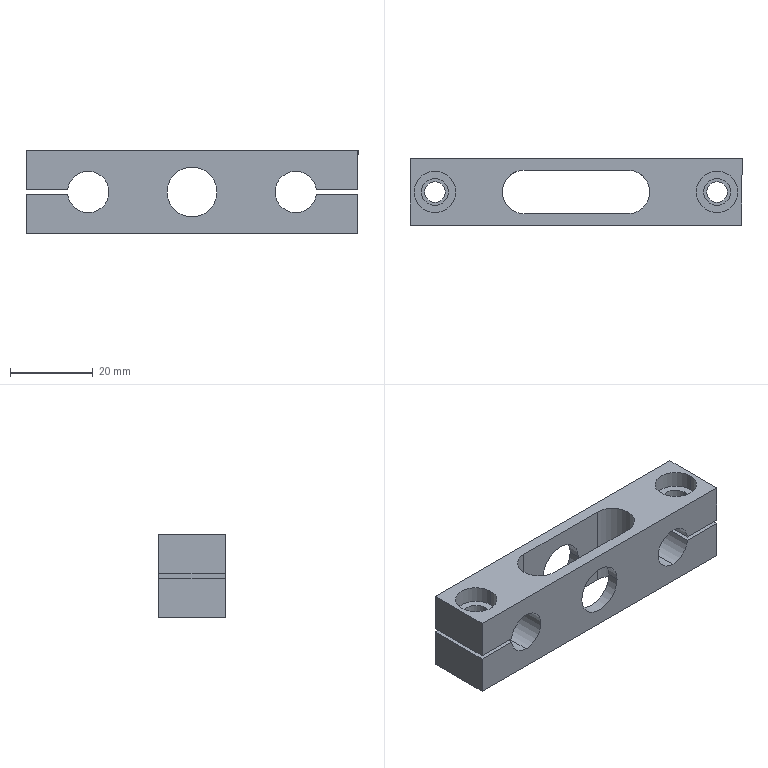Part | SolidWorks | features ICE 5, Extrusion 1, HoleWzd 1 | 1 solid | 41 faces | box 80 x 16 x 20 mm | volume 13796 mm3 | cylinder 25 | plane 16 | commonest cylinder face diameters 10 x10 5 x4 6.5 x4 12 x4 10.5 x3
STEP:
#1=CARTESIAN_POINT('',(-29.662,6.461,16.));
#2=VERTEX_POINT('',#1);
#3=CARTESIAN_POINT('',(-19.662,6.461,16.));
#4=VERTEX_POINT('',#3);
#5=CARTESIAN_POINT('',(-24.662,6.461,16.));
#6=DIRECTION('',(0.,0.,1.));
#7=DIRECTION('',(1.,0.,0.));
#8=AXIS2_PLACEMENT_3D('',#5,#6,#7);
#9=CIRCLE('',#8,5.);
#10=EDGE_CURVE('',#2,#4,#9,.T.);
#11=ORIENTED_EDGE('',*,*,#10,.F.);
#12=CARTESIAN_POINT('',(-29.662,6.461,20.));
#13=VERTEX_POINT('',#12);
#14=CARTESIAN_POINT('',(-29.662,6.461,16.));
#15=DIRECTION('',(0.,0.,1.));
#16=VECTOR('',#15,1000.);
#17=LINE('',#14,#16);
#18=EDGE_CURVE('',#2,#13,#17,.T.);
#19=ORIENTED_EDGE('',*,*,#18,.T.);
#20=CARTESIAN_POINT('',(-19.662,6.461,20.));
#21=VERTEX_POINT('',#20);
#22=CARTESIAN_POINT('',(-24.662,6.461,20.));
#23=DIRECTION('',(0.,0.,1.));
#24=DIRECTION('',(1.,0.,0.));
#25=AXIS2_PLACEMENT_3D('',#22,#23,#24);
#26=CIRCLE('',#25,5.);
#27=EDGE_CURVE('',#13,#21,#26,.T.);
#28=ORIENTED_EDGE('',*,*,#27,.T.);
#29=CARTESIAN_POINT('',(-19.662,6.461,16.));
#30=DIRECTION('',(0.,0.,1.));
#31=VECTOR('',#30,1000.);
#32=LINE('',#29,#31);
#33=EDGE_CURVE('',#4,#21,#32,.T.);
#34=ORIENTED_EDGE('',*,*,#33,.F.);
#35=EDGE_LOOP('',(#11,#19,#28,#34));
#36=FACE_OUTER_BOUND('',#35,.T.);
#37=CARTESIAN_POINT('',(-24.662,6.461,16.));
#38=DIRECTION('',(0.,0.,1.));
#39=DIRECTION('',(1.,0.,0.));
#40=AXIS2_PLACEMENT_3D('',#37,#38,#39);
#41=CYLINDRICAL_SURFACE('',#40,5.);
#42=ADVANCED_FACE('',(#36),#41,.F.);
#43=CARTESIAN_POINT('',(38.338,6.461,16.));
#44=VERTEX_POINT('',#43);
#45=CARTESIAN_POINT('',(48.338,6.461,16.));
#46=VERTEX_POINT('',#45);
#47=CARTESIAN_POINT('',(43.338,6.461,16.));
#48=DIRECTION('',(0.,0.,1.));
#49=DIRECTION('',(1.,0.,0.));
#50=AXIS2_PLACEMENT_3D('',#47,#48,#49);
#51=CIRCLE('',#50,5.);
#52=EDGE_CURVE('',#44,#46,#51,.T.);
#53=ORIENTED_EDGE('',*,*,#52,.F.);
#54=CARTESIAN_POINT('',(38.338,6.461,20.));
#55=VERTEX_POINT('',#54);
#56=CARTESIAN_POINT('',(38.338,6.461,16.));
#57=DIRECTION('',(0.,0.,1.));
#58=VECTOR('',#57,1000.);
#59=LINE('',#56,#58);
#60=EDGE_CURVE('',#44,#55,#59,.T.);
#61=ORIENTED_EDGE('',*,*,#60,.T.);
#62=CARTESIAN_POINT('',(48.338,6.461,20.));
#63=VERTEX_POINT('',#62);
#64=CARTESIAN_POINT('',(43.338,6.461,20.));
#65=DIRECTION('',(0.,0.,1.));
#66=DIRECTION('',(1.,0.,0.));
#67=AXIS2_PLACEMENT_3D('',#64,#65,#66);
#68=CIRCLE('',#67,5.);
#69=EDGE_CURVE('',#55,#63,#68,.T.);
#70=ORIENTED_EDGE('',*,*,#69,.T.);
#71=CARTESIAN_POINT('',(48.338,6.461,16.));
#72=DIRECTION('',(0.,0.,1.));
#73=VECTOR('',#72,1000.);
#74=LINE('',#71,#73);
#75=EDGE_CURVE('',#46,#63,#74,.T.);
#76=ORIENTED_EDGE('',*,*,#75,.F.);
#77=EDGE_LOOP('',(#53,#61,#70,#76));
#78=FACE_OUTER_BOUND('',#77,.T.);
#79=CARTESIAN_POINT('',(43.338,6.461,16.));
#80=DIRECTION('',(0.,0.,1.));
#81=DIRECTION('',(1.,0.,0.));
#82=AXIS2_PLACEMENT_3D('',#79,#80,#81);
#83=CYLINDRICAL_SURFACE('',#82,5.);
#84=ADVANCED_FACE('',(#78),#83,.F.);
#85=CARTESIAN_POINT('',(45.838,6.461,0.));
#86=VERTEX_POINT('',#85);
#87=CARTESIAN_POINT('',(40.838,6.461,0.));
#88=VERTEX_POINT('',#87);
#89=CARTESIAN_POINT('',(43.338,6.461,0.));
#90=DIRECTION('',(0.,0.,-1.));
#91=DIRECTION('',(-1.,0.,0.));
#92=AXIS2_PLACEMENT_3D('',#89,#90,#91);
#93=CIRCLE('',#92,2.5);
#94=EDGE_CURVE('',#86,#88,#93,.T.);
#95=ORIENTED_EDGE('',*,*,#94,.T.);
#96=CARTESIAN_POINT('',(40.838,6.461,9.5));
#97=VERTEX_POINT('',#96);
#98=CARTESIAN_POINT('',(40.838,6.461,9.5));
#99=DIRECTION('',(0.,0.,1.));
#100=VECTOR('',#99,1000.);
#101=LINE('',#98,#100);
#102=EDGE_CURVE('',#88,#97,#101,.T.);
#103=ORIENTED_EDGE('',*,*,#102,.T.);
#104=CARTESIAN_POINT('',(45.838,6.461,9.5));
#105=VERTEX_POINT('',#104);
#106=CARTESIAN_POINT('',(43.338,6.461,9.5));
#107=DIRECTION('',(0.,0.,1.));
#108=DIRECTION('',(1.,0.,0.));
#109=AXIS2_PLACEMENT_3D('',#106,#107,#108);
#110=CIRCLE('',#109,2.5);
#111=EDGE_CURVE('',#97,#105,#110,.T.);
#112=ORIENTED_EDGE('',*,*,#111,.T.);
#113=CARTESIAN_POINT('',(45.838,6.461,9.5));
#114=DIRECTION('',(0.,0.,1.));
#115=VECTOR('',#114,1000.);
#116=LINE('',#113,#115);
#117=EDGE_CURVE('',#86,#105,#116,.T.);
#118=ORIENTED_EDGE('',*,*,#117,.F.);
#119=EDGE_LOOP('',(#95,#103,#112,#118));
#120=FACE_OUTER_BOUND('',#119,.T.);
#121=CARTESIAN_POINT('',(43.338,6.461,9.5));
#122=DIRECTION('',(0.,0.,1.));
#123=DIRECTION('',(1.,0.,0.));
#124=AXIS2_PLACEMENT_3D('',#121,#122,#123);
#125=CYLINDRICAL_SURFACE('',#124,2.5);
#126=ADVANCED_FACE('',(#120),#125,.F.);
#127=CARTESIAN_POINT('',(-22.162,6.461,0.));
#128=VERTEX_POINT('',#127);
#129=CARTESIAN_POINT('',(-27.162,6.461,0.));
#130=VERTEX_POINT('',#129);
#131=CARTESIAN_POINT('',(-24.662,6.461,0.));
#132=DIRECTION('',(0.,0.,-1.));
#133=DIRECTION('',(-1.,0.,0.));
#134=AXIS2_PLACEMENT_3D('',#131,#132,#133);
#135=CIRCLE('',#134,2.5);
#136=EDGE_CURVE('',#128,#130,#135,.T.);
#137=ORIENTED_EDGE('',*,*,#136,.T.);
#138=CARTESIAN_POINT('',(-27.162,6.461,9.5));
#139=VERTEX_POINT('',#138);
#140=CARTESIAN_POINT('',(-27.162,6.461,9.5));
#141=DIRECTION('',(0.,0.,1.));
#142=VECTOR('',#141,1000.);
#143=LINE('',#140,#142);
#144=EDGE_CURVE('',#130,#139,#143,.T.);
#145=ORIENTED_EDGE('',*,*,#144,.T.);
#146=CARTESIAN_POINT('',(-22.162,6.461,9.5));
#147=VERTEX_POINT('',#146);
#148=CARTESIAN_POINT('',(-24.662,6.461,9.5));
#149=DIRECTION('',(0.,0.,1.));
#150=DIRECTION('',(1.,0.,0.));
#151=AXIS2_PLACEMENT_3D('',#148,#149,#150);
#152=CIRCLE('',#151,2.5);
#153=EDGE_CURVE('',#139,#147,#152,.T.);
#154=ORIENTED_EDGE('',*,*,#153,.T.);
#155=CARTESIAN_POINT('',(-22.162,6.461,9.5));
#156=DIRECTION('',(0.,0.,1.));
#157=VECTOR('',#156,1000.);
#158=LINE('',#155,#157);
#159=EDGE_CURVE('',#128,#147,#158,.T.);
#160=ORIENTED_EDGE('',*,*,#159,.F.);
#161=EDGE_LOOP('',(#137,#145,#154,#160));
#162=FACE_OUTER_BOUND('',#161,.T.);
#163=CARTESIAN_POINT('',(-24.662,6.461,9.5));
#164=DIRECTION('',(0.,0.,1.));
#165=DIRECTION('',(1.,0.,0.));
#166=AXIS2_PLACEMENT_3D('',#163,#164,#165);
#167=CYLINDRICAL_SURFACE('',#166,2.5);
#168=ADVANCED_FACE('',(#162),#167,.F.);
#169=CARTESIAN_POINT('',(15.338,1.211,10.));
#170=VERTEX_POINT('',#169);
#171=CARTESIAN_POINT('',(3.338,1.211,10.));
#172=VERTEX_POINT('',#171);
#173=CARTESIAN_POINT('',(9.338,1.211,10.));
#174=DIRECTION('',(0.,1.,0.));
#175=DIRECTION('',(0.,0.,1.));
#176=AXIS2_PLACEMENT_3D('',#173,#174,#175);
#177=CIRCLE('',#176,6.);
#178=EDGE_CURVE('',#170,#172,#177,.T.);
#179=ORIENTED_EDGE('',*,*,#178,.T.);
#180=CARTESIAN_POINT('',(3.338,-1.539,10.));
#181=VERTEX_POINT('',#180);
#182=CARTESIAN_POINT('',(3.338,28.211,10.));
#183=DIRECTION('',(0.,-1.,0.));
#184=VECTOR('',#183,1000.);
#185=LINE('',#182,#184);
#186=EDGE_CURVE('',#172,#181,#185,.T.);
#187=ORIENTED_EDGE('',*,*,#186,.T.);
#188=CARTESIAN_POINT('',(15.338,-1.539,10.));
#189=VERTEX_POINT('',#188);
#190=CARTESIAN_POINT('',(9.338,-1.539,10.));
#191=DIRECTION('',(0.,1.,0.));
#192=DIRECTION('',(0.,0.,1.));
#193=AXIS2_PLACEMENT_3D('',#190,#191,#192);
#194=CIRCLE('',#193,6.);
#195=EDGE_CURVE('',#189,#181,#194,.T.);
#196=ORIENTED_EDGE('',*,*,#195,.F.);
#197=CARTESIAN_POINT('',(15.338,28.211,10.));
#198=DIRECTION('',(0.,-1.,0.));
#199=VECTOR('',#198,1000.);
#200=LINE('',#197,#199);
#201=EDGE_CURVE('',#170,#189,#200,.T.);
#202=ORIENTED_EDGE('',*,*,#201,.F.);
#203=EDGE_LOOP('',(#179,#187,#196,#202));
#204=FACE_OUTER_BOUND('',#203,.T.);
#205=CARTESIAN_POINT('',(9.338,28.211,10.));
#206=DIRECTION('',(0.,-1.,0.));
#207=DIRECTION('',(1.,0.,0.));
#208=AXIS2_PLACEMENT_3D('',#205,#206,#207);
#209=CYLINDRICAL_SURFACE('',#208,6.);
#210=ADVANCED_FACE('',(#204),#209,.F.);
#211=CARTESIAN_POINT('',(3.338,14.461,10.));
#212=VERTEX_POINT('',#211);
#213=CARTESIAN_POINT('',(15.338,14.461,10.));
#214=VERTEX_POINT('',#213);
#215=CARTESIAN_POINT('',(9.338,14.461,10.));
#216=DIRECTION('',(0.,-1.,0.));
#217=DIRECTION('',(0.,0.,-1.));
#218=AXIS2_PLACEMENT_3D('',#215,#216,#217);
#219=CIRCLE('',#218,6.);
#220=EDGE_CURVE('',#212,#214,#219,.T.);
#221=ORIENTED_EDGE('',*,*,#220,.F.);
#222=CARTESIAN_POINT('',(3.338,11.711,10.));
#223=VERTEX_POINT('',#222);
#224=CARTESIAN_POINT('',(3.338,28.211,10.));
#225=DIRECTION('',(0.,-1.,0.));
#226=VECTOR('',#225,1000.);
#227=LINE('',#224,#226);
#228=EDGE_CURVE('',#212,#223,#227,.T.);
#229=ORIENTED_EDGE('',*,*,#228,.T.);
#230=CARTESIAN_POINT('',(15.338,11.711,10.));
#231=VERTEX_POINT('',#230);
#232=CARTESIAN_POINT('',(9.338,11.711,10.));
#233=DIRECTION('',(0.,-1.,0.));
#234=DIRECTION('',(0.,0.,-1.));
#235=AXIS2_PLACEMENT_3D('',#232,#233,#234);
#236=CIRCLE('',#235,6.);
#237=EDGE_CURVE('',#223,#231,#236,.T.);
#238=ORIENTED_EDGE('',*,*,#237,.T.);
#239=CARTESIAN_POINT('',(15.338,28.211,10.));
#240=DIRECTION('',(0.,-1.,0.));
#241=VECTOR('',#240,1000.);
#242=LINE('',#239,#241);
#243=EDGE_CURVE('',#214,#231,#242,.T.);
#244=ORIENTED_EDGE('',*,*,#243,.F.);
#245=EDGE_LOOP('',(#221,#229,#238,#244));
#246=FACE_OUTER_BOUND('',#245,.T.);
#247=CARTESIAN_POINT('',(9.338,28.211,10.));
#248=DIRECTION('',(0.,-1.,0.));
#249=DIRECTION('',(1.,0.,0.));
#250=AXIS2_PLACEMENT_3D('',#247,#248,#249);
#251=CYLINDRICAL_SURFACE('',#250,6.);
#252=ADVANCED_FACE('',(#246),#251,.F.);
#253=CARTESIAN_POINT('',(-15.662,14.461,15.));
#254=VERTEX_POINT('',#253);
#255=CARTESIAN_POINT('',(-20.637,14.461,10.5));
#256=VERTEX_POINT('',#255);
#257=CARTESIAN_POINT('',(-15.662,14.461,10.));
#258=DIRECTION('',(0.,-1.,0.));
#259=DIRECTION('',(0.,0.,-1.));
#260=AXIS2_PLACEMENT_3D('',#257,#258,#259);
#261=CIRCLE('',#260,5.);
#262=EDGE_CURVE('',#254,#256,#261,.T.);
#263=ORIENTED_EDGE('',*,*,#262,.F.);
#264=CARTESIAN_POINT('',(-15.662,-1.539,15.));
#265=VERTEX_POINT('',#264);
#266=CARTESIAN_POINT('',(-15.662,18.461,15.));
#267=DIRECTION('',(0.,-1.,0.));
#268=VECTOR('',#267,1000.);
#269=LINE('',#266,#268);
#270=EDGE_CURVE('',#254,#265,#269,.T.);
#271=ORIENTED_EDGE('',*,*,#270,.T.);
#272=CARTESIAN_POINT('',(-20.637,-1.539,10.5));
#273=VERTEX_POINT('',#272);
#274=CARTESIAN_POINT('',(-15.662,-1.539,10.));
#275=DIRECTION('',(0.,-1.,0.));
#276=DIRECTION('',(0.,0.,-1.));
#277=AXIS2_PLACEMENT_3D('',#274,#275,#276);
#278=CIRCLE('',#277,5.);
#279=EDGE_CURVE('',#265,#273,#278,.T.);
#280=ORIENTED_EDGE('',*,*,#279,.T.);
#281=CARTESIAN_POINT('',(-20.637,18.461,10.5));
#282=DIRECTION('',(0.,1.,0.));
#283=VECTOR('',#282,1000.);
#284=LINE('',#281,#283);
#285=EDGE_CURVE('',#273,#256,#284,.T.);
#286=ORIENTED_EDGE('',*,*,#285,.T.);
#287=EDGE_LOOP('',(#263,#271,#280,#286));
#288=FACE_OUTER_BOUND('',#287,.T.);
#289=CARTESIAN_POINT('',(-15.662,18.461,10.));
#290=DIRECTION('',(0.,-1.,0.));
#291=DIRECTION('',(0.,0.,-1.));
#292=AXIS2_PLACEMENT_3D('',#289,#290,#291);
#293=CYLINDRICAL_SURFACE('',#292,5.);
#294=ADVANCED_FACE('',(#288),#293,.F.);
#295=ORIENTED_EDGE('',*,*,#270,.F.);
#296=CARTESIAN_POINT('',(-15.662,14.461,5.));
#297=VERTEX_POINT('',#296);
#298=CARTESIAN_POINT('',(-15.662,14.461,10.));
#299=DIRECTION('',(0.,-1.,0.));
#300=DIRECTION('',(0.,0.,-1.));
#301=AXIS2_PLACEMENT_3D('',#298,#299,#300);
#302=CIRCLE('',#301,5.);
#303=EDGE_CURVE('',#297,#254,#302,.T.);
#304=ORIENTED_EDGE('',*,*,#303,.F.);
#305=CARTESIAN_POINT('',(-15.662,-1.539,5.));
#306=VERTEX_POINT('',#305);
#307=CARTESIAN_POINT('',(-15.662,18.461,5.));
#308=DIRECTION('',(0.,-1.,0.));
#309=VECTOR('',#308,1000.);
#310=LINE('',#307,#309);
#311=EDGE_CURVE('',#297,#306,#310,.T.);
#312=ORIENTED_EDGE('',*,*,#311,.T.);
#313=CARTESIAN_POINT('',(-15.662,-1.539,10.));
#314=DIRECTION('',(0.,-1.,0.));
#315=DIRECTION('',(0.,0.,-1.));
#316=AXIS2_PLACEMENT_3D('',#313,#314,#315);
#317=CIRCLE('',#316,5.);
#318=EDGE_CURVE('',#306,#265,#317,.T.);
#319=ORIENTED_EDGE('',*,*,#318,.T.);
#320=EDGE_LOOP('',(#295,#304,#312,#319));
#321=FACE_OUTER_BOUND('',#320,.T.);
#322=CARTESIAN_POINT('',(-15.662,18.461,10.));
#323=DIRECTION('',(0.,-1.,0.));
#324=DIRECTION('',(0.,0.,-1.));
#325=AXIS2_PLACEMENT_3D('',#322,#323,#324);
#326=CYLINDRICAL_SURFACE('',#325,5.);
#327=ADVANCED_FACE('',(#321),#326,.F.);
#328=CARTESIAN_POINT('',(34.338,14.461,15.));
#329=VERTEX_POINT('',#328);
#330=CARTESIAN_POINT('',(34.338,14.461,5.));
#331=VERTEX_POINT('',#330);
#332=CARTESIAN_POINT('',(34.338,14.461,10.));
#333=DIRECTION('',(0.,-1.,0.));
#334=DIRECTION('',(0.,0.,-1.));
#335=AXIS2_PLACEMENT_3D('',#332,#333,#334);
#336=CIRCLE('',#335,5.);
#337=EDGE_CURVE('',#329,#331,#336,.T.);
#338=ORIENTED_EDGE('',*,*,#337,.F.);
#339=CARTESIAN_POINT('',(34.338,-1.539,15.));
#340=VERTEX_POINT('',#339);
#341=CARTESIAN_POINT('',(34.338,18.461,15.));
#342=DIRECTION('',(0.,-1.,0.));
#343=VECTOR('',#342,1000.);
#344=LINE('',#341,#343);
#345=EDGE_CURVE('',#329,#340,#344,.T.);
#346=ORIENTED_EDGE('',*,*,#345,.T.);
#347=CARTESIAN_POINT('',(34.338,-1.539,5.));
#348=VERTEX_POINT('',#347);
#349=CARTESIAN_POINT('',(34.338,-1.539,10.));
#350=DIRECTION('',(0.,-1.,0.));
#351=DIRECTION('',(0.,0.,-1.));
#352=AXIS2_PLACEMENT_3D('',#349,#350,#351);
#353=CIRCLE('',#352,5.);
#354=EDGE_CURVE('',#340,#348,#353,.T.);
#355=ORIENTED_EDGE('',*,*,#354,.T.);
#356=CARTESIAN_POINT('',(34.338,18.461,5.));
#357=DIRECTION('',(0.,-1.,0.));
#358=VECTOR('',#357,1000.);
#359=LINE('',#356,#358);
#360=EDGE_CURVE('',#331,#348,#359,.T.);
#361=ORIENTED_EDGE('',*,*,#360,.F.);
#362=EDGE_LOOP('',(#338,#346,#355,#361));
#363=FACE_OUTER_BOUND('',#362,.T.);
#364=CARTESIAN_POINT('',(34.338,18.461,10.));
#365=DIRECTION('',(0.,-1.,0.));
#366=DIRECTION('',(0.,0.,-1.));
#367=AXIS2_PLACEMENT_3D('',#364,#365,#366);
#368=CYLINDRICAL_SURFACE('',#367,5.);
#369=ADVANCED_FACE('',(#363),#368,.F.);
#370=CARTESIAN_POINT('',(39.313,14.461,9.5));
#371=VERTEX_POINT('',#370);
#372=CARTESIAN_POINT('',(34.338,14.461,10.));
#373=DIRECTION('',(0.,-1.,0.));
#374=DIRECTION('',(0.,0.,-1.));
#375=AXIS2_PLACEMENT_3D('',#372,#373,#374);
#376=CIRCLE('',#375,5.);
#377=EDGE_CURVE('',#331,#371,#376,.T.);
#378=ORIENTED_EDGE('',*,*,#377,.F.);
#379=ORIENTED_EDGE('',*,*,#360,.T.);
#380=CARTESIAN_POINT('',(39.313,-1.539,9.5));
#381=VERTEX_POINT('',#380);
#382=CARTESIAN_POINT('',(34.338,-1.539,10.));
#383=DIRECTION('',(0.,-1.,0.));
#384=DIRECTION('',(0.,0.,-1.));
#385=AXIS2_PLACEMENT_3D('',#382,#383,#384);
#386=CIRCLE('',#385,5.);
#387=EDGE_CURVE('',#348,#381,#386,.T.);
#388=ORIENTED_EDGE('',*,*,#387,.T.);
#389=CARTESIAN_POINT('',(39.313,18.461,9.5));
#390=DIRECTION('',(0.,1.,0.));
#391=VECTOR('',#390,1000.);
#392=LINE('',#389,#391);
#393=EDGE_CURVE('',#381,#371,#392,.T.);
#394=ORIENTED_EDGE('',*,*,#393,.T.);
#395=EDGE_LOOP('',(#378,#379,#388,#394));
#396=FACE_OUTER_BOUND('',#395,.T.);
#397=CARTESIAN_POINT('',(34.338,18.461,10.));
#398=DIRECTION('',(0.,-1.,0.));
#399=DIRECTION('',(0.,0.,-1.));
#400=AXIS2_PLACEMENT_3D('',#397,#398,#399);
#401=CYLINDRICAL_SURFACE('',#400,5.);
#402=ADVANCED_FACE('',(#396),#401,.F.);
#403=CARTESIAN_POINT('',(-3.162,11.711,20.));
#404=VERTEX_POINT('',#403);
#405=CARTESIAN_POINT('',(-8.412,6.461,20.));
#406=VERTEX_POINT('',#405);
#407=CARTESIAN_POINT('',(-3.162,6.461,20.));
#408=DIRECTION('',(0.,0.,1.));
#409=DIRECTION('',(1.,0.,0.));
#410=AXIS2_PLACEMENT_3D('',#407,#408,#409);
#411=CIRCLE('',#410,5.25);
#412=EDGE_CURVE('',#404,#406,#411,.T.);
#413=ORIENTED_EDGE('',*,*,#412,.T.);
#414=CARTESIAN_POINT('',(-8.412,6.461,0.));
#415=VERTEX_POINT('',#414);
#416=CARTESIAN_POINT('',(-8.412,6.461,20.));
#417=DIRECTION('',(0.,0.,-1.));
#418=VECTOR('',#417,1000.);
#419=LINE('',#416,#418);
#420=EDGE_CURVE('',#406,#415,#419,.T.);
#421=ORIENTED_EDGE('',*,*,#420,.T.);
#422=CARTESIAN_POINT('',(-3.162,11.711,0.));
#423=VERTEX_POINT('',#422);
#424=CARTESIAN_POINT('',(-3.162,6.461,0.));
#425=DIRECTION('',(0.,0.,1.));
#426=DIRECTION('',(1.,0.,0.));
#427=AXIS2_PLACEMENT_3D('',#424,#425,#426);
#428=CIRCLE('',#427,5.25);
#429=EDGE_CURVE('',#423,#415,#428,.T.);
#430=ORIENTED_EDGE('',*,*,#429,.F.);
#431=CARTESIAN_POINT('',(-3.162,11.711,20.));
#432=DIRECTION('',(0.,0.,-1.));
#433=VECTOR('',#432,1000.);
#434=LINE('',#431,#433);
#435=EDGE_CURVE('',#404,#423,#434,.T.);
#436=ORIENTED_EDGE('',*,*,#435,.F.);
#437=EDGE_LOOP('',(#413,#421,#430,#436));
#438=FACE_OUTER_BOUND('',#437,.T.);
#439=CARTESIAN_POINT('',(-3.162,6.461,20.));
#440=DIRECTION('',(0.,0.,-1.));
#441=DIRECTION('',(-1.,0.,0.));
#442=AXIS2_PLACEMENT_3D('',#439,#440,#441);
#443=CYLINDRICAL_SURFACE('',#442,5.25);
#444=ADVANCED_FACE('',(#438),#443,.F.);
#445=CARTESIAN_POINT('',(46.588,6.461,16.));
#446=VERTEX_POINT('',#445);
#447=CARTESIAN_POINT('',(40.088,6.461,16.));
#448=VERTEX_POINT('',#447);
#449=CARTESIAN_POINT('',(43.338,6.461,16.));
#450=DIRECTION('',(0.,0.,-1.));
#451=DIRECTION('',(1.,0.,0.));
#452=AXIS2_PLACEMENT_3D('',#449,#450,#451);
#453=CIRCLE('',#452,3.25);
#454=EDGE_CURVE('',#446,#448,#453,.T.);
#455=ORIENTED_EDGE('',*,*,#454,.F.);
#456=CARTESIAN_POINT('',(46.588,6.461,10.5));
#457=VERTEX_POINT('',#456);
#458=CARTESIAN_POINT('',(46.588,6.461,40.5));
#459=DIRECTION('',(0.,0.,-1.));
#460=VECTOR('',#459,1000.);
#461=LINE('',#458,#460);
#462=EDGE_CURVE('',#446,#457,#461,.T.);
#463=ORIENTED_EDGE('',*,*,#462,.T.);
#464=CARTESIAN_POINT('',(40.088,6.461,10.5));
#465=VERTEX_POINT('',#464);
#466=CARTESIAN_POINT('',(43.338,6.461,10.5));
#467=DIRECTION('',(0.,0.,-1.));
#468=DIRECTION('',(-1.,0.,0.));
#469=AXIS2_PLACEMENT_3D('',#466,#467,#468);
#470=CIRCLE('',#469,3.25);
#471=EDGE_CURVE('',#457,#465,#470,.T.);
#472=ORIENTED_EDGE('',*,*,#471,.T.);
#473=CARTESIAN_POINT('',(40.088,6.461,40.5));
#474=DIRECTION('',(0.,0.,-1.));
#475=VECTOR('',#474,1000.);
#476=LINE('',#473,#475);
#477=EDGE_CURVE('',#448,#465,#476,.T.);
#478=ORIENTED_EDGE('',*,*,#477,.F.);
#479=EDGE_LOOP('',(#455,#463,#472,#478));
#480=FACE_OUTER_BOUND('',#479,.T.);
#481=CARTESIAN_POINT('',(43.338,6.461,40.5));
#482=DIRECTION('',(0.,0.,-1.));
#483=DIRECTION('',(-1.,0.,0.));
#484=AXIS2_PLACEMENT_3D('',#481,#482,#483);
#485=CYLINDRICAL_SURFACE('',#484,3.25);
#486=ADVANCED_FACE('',(#480),#485,.F.);
#487=CARTESIAN_POINT('',(-21.412,6.461,16.));
#488=VERTEX_POINT('',#487);
#489=CARTESIAN_POINT('',(-27.912,6.461,16.));
#490=VERTEX_POINT('',#489);
#491=CARTESIAN_POINT('',(-24.662,6.461,16.));
#492=DIRECTION('',(0.,0.,-1.));
#493=DIRECTION('',(1.,0.,0.));
#494=AXIS2_PLACEMENT_3D('',#491,#492,#493);
#495=CIRCLE('',#494,3.25);
#496=EDGE_CURVE('',#488,#490,#495,.T.);
#497=ORIENTED_EDGE('',*,*,#496,.F.);
#498=CARTESIAN_POINT('',(-21.412,6.461,10.5));
#499=VERTEX_POINT('',#498);
#500=CARTESIAN_POINT('',(-21.412,6.461,40.5));
#501=DIRECTION('',(0.,0.,-1.));
#502=VECTOR('',#501,1000.);
#503=LINE('',#500,#502);
#504=EDGE_CURVE('',#488,#499,#503,.T.);
#505=ORIENTED_EDGE('',*,*,#504,.T.);
#506=CARTESIAN_POINT('',(-27.912,6.461,10.5));
#507=VERTEX_POINT('',#506);
#508=CARTESIAN_POINT('',(-24.662,6.461,10.5));
#509=DIRECTION('',(0.,0.,-1.));
#510=DIRECTION('',(-1.,0.,0.));
#511=AXIS2_PLACEMENT_3D('',#508,#509,#510);
#512=CIRCLE('',#511,3.25);
#513=EDGE_CURVE('',#499,#507,#512,.T.);
#514=ORIENTED_EDGE('',*,*,#513,.T.);
#515=CARTESIAN_POINT('',(-27.912,6.461,40.5));
#516=DIRECTION('',(0.,0.,-1.));
#517=VECTOR('',#516,1000.);
#518=LINE('',#515,#517);
#519=EDGE_CURVE('',#490,#507,#518,.T.);
#520=ORIENTED_EDGE('',*,*,#519,.F.);
#521=EDGE_LOOP('',(#497,#505,#514,#520));
#522=FACE_OUTER_BOUND('',#521,.T.);
#523=CARTESIAN_POINT('',(-24.662,6.461,40.5));
#524=DIRECTION('',(0.,0.,-1.));
#525=DIRECTION('',(-1.,0.,0.));
#526=AXIS2_PLACEMENT_3D('',#523,#524,#525);
#527=CYLINDRICAL_SURFACE('',#526,3.25);
#528=ADVANCED_FACE('',(#522),#527,.F.);
#529=ORIENTED_EDGE('',*,*,#504,.F.);
#530=CARTESIAN_POINT('',(-24.662,6.461,16.));
#531=DIRECTION('',(0.,0.,-1.));
#532=DIRECTION('',(1.,0.,0.));
#533=AXIS2_PLACEMENT_3D('',#530,#531,#532);
#534=CIRCLE('',#533,3.25);
#535=EDGE_CURVE('',#490,#488,#534,.T.);
#536=ORIENTED_EDGE('',*,*,#535,.F.);
#537=ORIENTED_EDGE('',*,*,#519,.T.);
#538=CARTESIAN_POINT('',(-24.662,6.461,10.5));
#539=DIRECTION('',(0.,0.,-1.));
#540=DIRECTION('',(-1.,0.,0.));
#541=AXIS2_PLACEMENT_3D('',#538,#539,#540);
#542=CIRCLE('',#541,3.25);
#543=EDGE_CURVE('',#507,#499,#542,.T.);
#544=ORIENTED_EDGE('',*,*,#543,.T.);
#545=EDGE_LOOP('',(#529,#536,#537,#544));
#546=FACE_OUTER_BOUND('',#545,.T.);
#547=CARTESIAN_POINT('',(-24.662,6.461,40.5));
#548=DIRECTION('',(0.,0.,-1.));
#549=DIRECTION('',(-1.,0.,0.));
#550=AXIS2_PLACEMENT_3D('',#547,#548,#549);
#551=CYLINDRICAL_SURFACE('',#550,3.25);
#552=ADVANCED_FACE('',(#546),#551,.F.);
#553=ORIENTED_EDGE('',*,*,#462,.F.);
#554=CARTESIAN_POINT('',(43.338,6.461,16.));
#555=DIRECTION('',(0.,0.,-1.));
#556=DIRECTION('',(1.,0.,0.));
#557=AXIS2_PLACEMENT_3D('',#554,#555,#556);
#558=CIRCLE('',#557,3.25);
#559=EDGE_CURVE('',#448,#446,#558,.T.);
#560=ORIENTED_EDGE('',*,*,#559,.F.);
#561=ORIENTED_EDGE('',*,*,#477,.T.);
#562=CARTESIAN_POINT('',(43.338,6.461,10.5));
#563=DIRECTION('',(0.,0.,-1.));
#564=DIRECTION('',(-1.,0.,0.));
#565=AXIS2_PLACEMENT_3D('',#562,#563,#564);
#566=CIRCLE('',#565,3.25);
#567=EDGE_CURVE('',#465,#457,#566,.T.);
#568=ORIENTED_EDGE('',*,*,#567,.T.);
#569=EDGE_LOOP('',(#553,#560,#561,#568));
#570=FACE_OUTER_BOUND('',#569,.T.);
#571=CARTESIAN_POINT('',(43.338,6.461,40.5));
#572=DIRECTION('',(0.,0.,-1.));
#573=DIRECTION('',(-1.,0.,0.));
#574=AXIS2_PLACEMENT_3D('',#571,#572,#573);
#575=CYLINDRICAL_SURFACE('',#574,3.25);
#576=ADVANCED_FACE('',(#570),#575,.F.);
#577=CARTESIAN_POINT('',(-30.662,-1.539,9.5));
#578=VERTEX_POINT('',#577);
#579=CARTESIAN_POINT('',(-30.662,-1.539,0.));
#580=VERTEX_POINT('',#579);
#581=CARTESIAN_POINT('',(-30.662,-1.539,20.));
#582=DIRECTION('',(0.,0.,-1.));
#583=VECTOR('',#582,1000.);
#584=LINE('',#581,#583);
#585=EDGE_CURVE('',#578,#580,#584,.T.);
#586=ORIENTED_EDGE('',*,*,#585,.F.);
#587=CARTESIAN_POINT('',(-30.662,14.461,9.5));
#588=VERTEX_POINT('',#587);
#589=CARTESIAN_POINT('',(-30.662,-1.539,9.5));
#590=DIRECTION('',(0.,1.,0.));
#591=VECTOR('',#590,1000.);
#592=LINE('',#589,#591);
#593=EDGE_CURVE('',#578,#588,#592,.T.);
#594=ORIENTED_EDGE('',*,*,#593,.T.);
#595=CARTESIAN_POINT('',(-30.662,14.461,0.));
#596=VERTEX_POINT('',#595);
#597=CARTESIAN_POINT('',(-30.662,14.461,20.));
#598=DIRECTION('',(0.,0.,-1.));
#599=VECTOR('',#598,1000.);
#600=LINE('',#597,#599);
#601=EDGE_CURVE('',#588,#596,#600,.T.);
#602=ORIENTED_EDGE('',*,*,#601,.T.);
#603=CARTESIAN_POINT('',(-30.662,-1.539,0.));
#604=DIRECTION('',(0.,-1.,0.));
#605=VECTOR('',#604,1000.);
#606=LINE('',#603,#605);
#607=EDGE_CURVE('',#596,#580,#606,.T.);
#608=ORIENTED_EDGE('',*,*,#607,.T.);
#609=EDGE_LOOP('',(#586,#594,#602,#608));
#610=FACE_OUTER_BOUND('',#609,.T.);
#611=CARTESIAN_POINT('',(-30.662,-1.539,20.));
#612=DIRECTION('',(1.,0.,0.));
#613=DIRECTION('',(0.,0.,-1.));
#614=AXIS2_PLACEMENT_3D('',#611,#612,#613);
#615=PLANE('',#614);
#616=ADVANCED_FACE('',(#610),#615,.F.);
#617=CARTESIAN_POINT('',(49.338,-1.539,20.));
#618=VERTEX_POINT('',#617);
#619=CARTESIAN_POINT('',(49.338,-1.539,10.5));
#620=VERTEX_POINT('',#619);
#621=CARTESIAN_POINT('',(49.338,-1.539,20.));
#622=DIRECTION('',(0.,0.,-1.));
#623=VECTOR('',#622,1000.);
#624=LINE('',#621,#623);
#625=EDGE_CURVE('',#618,#620,#624,.T.);
#626=ORIENTED_EDGE('',*,*,#625,.T.);
#627=CARTESIAN_POINT('',(49.338,14.461,10.5));
#628=VERTEX_POINT('',#627);
#629=CARTESIAN_POINT('',(49.338,-1.539,10.5));
#630=DIRECTION('',(0.,1.,0.));
#631=VECTOR('',#630,1000.);
#632=LINE('',#629,#631);
#633=EDGE_CURVE('',#620,#628,#632,.T.);
#634=ORIENTED_EDGE('',*,*,#633,.T.);
#635=CARTESIAN_POINT('',(49.338,14.461,20.));
#636=VERTEX_POINT('',#635);
#637=CARTESIAN_POINT('',(49.338,14.461,20.));
#638=DIRECTION('',(0.,0.,-1.));
#639=VECTOR('',#638,1000.);
#640=LINE('',#637,#639);
#641=EDGE_CURVE('',#636,#628,#640,.T.);
#642=ORIENTED_EDGE('',*,*,#641,.F.);
#643=CARTESIAN_POINT('',(49.338,-1.539,20.));
#644=DIRECTION('',(0.,1.,0.));
#645=VECTOR('',#644,1000.);
#646=LINE('',#643,#645);
#647=EDGE_CURVE('',#618,#636,#646,.T.);
#648=ORIENTED_EDGE('',*,*,#647,.F.);
#649=EDGE_LOOP('',(#626,#634,#642,#648));
#650=FACE_OUTER_BOUND('',#649,.T.);
#651=CARTESIAN_POINT('',(49.338,-1.539,20.));
#652=DIRECTION('',(-1.,0.,0.));
#653=DIRECTION('',(0.,0.,1.));
#654=AXIS2_PLACEMENT_3D('',#651,#652,#653);
#655=PLANE('',#654);
#656=ADVANCED_FACE('',(#650),#655,.F.);
#657=CARTESIAN_POINT('',(-24.662,6.461,20.));
#658=DIRECTION('',(0.,0.,1.));
#659=DIRECTION('',(1.,0.,0.));
#660=AXIS2_PLACEMENT_3D('',#657,#658,#659);
#661=CIRCLE('',#660,5.);
#662=EDGE_CURVE('',#21,#13,#661,.T.);
#663=ORIENTED_EDGE('',*,*,#662,.F.);
#664=ORIENTED_EDGE('',*,*,#27,.F.);
#665=EDGE_LOOP('',(#663,#664));
#666=FACE_BOUND('',#665,.T.);
#667=CARTESIAN_POINT('',(43.338,6.461,20.));
#668=DIRECTION('',(0.,0.,1.));
#669=DIRECTION('',(1.,0.,0.));
#670=AXIS2_PLACEMENT_3D('',#667,#668,#669);
#671=CIRCLE('',#670,5.);
#672=EDGE_CURVE('',#63,#55,#671,.T.);
#673=ORIENTED_EDGE('',*,*,#672,.F.);
#674=ORIENTED_EDGE('',*,*,#69,.F.);
#675=EDGE_LOOP('',(#673,#674));
#676=FACE_BOUND('',#675,.T.);
#677=CARTESIAN_POINT('',(-30.662,14.461,20.));
#678=VERTEX_POINT('',#677);
#679=CARTESIAN_POINT('',(-30.662,-1.539,20.));
#680=VERTEX_POINT('',#679);
#681=CARTESIAN_POINT('',(-30.662,-1.539,20.));
#682=DIRECTION('',(0.,-1.,0.));
#683=VECTOR('',#682,1000.);
#684=LINE('',#681,#683);
#685=EDGE_CURVE('',#678,#680,#684,.T.);
#686=ORIENTED_EDGE('',*,*,#685,.T.);
#687=CARTESIAN_POINT('',(-30.662,-1.539,20.));
#688=DIRECTION('',(1.,0.,0.));
#689=VECTOR('',#688,1000.);
#690=LINE('',#687,#689);
#691=EDGE_CURVE('',#680,#618,#690,.T.);
#692=ORIENTED_EDGE('',*,*,#691,.T.);
#693=ORIENTED_EDGE('',*,*,#647,.T.);
#694=CARTESIAN_POINT('',(-30.662,14.461,20.));
#695=DIRECTION('',(-1.,0.,0.));
#696=VECTOR('',#695,1000.);
#697=LINE('',#694,#696);
#698=EDGE_CURVE('',#636,#678,#697,.T.);
#699=ORIENTED_EDGE('',*,*,#698,.T.);
#700=EDGE_LOOP('',(#686,#692,#693,#699));
#701=FACE_OUTER_BOUND('',#700,.T.);
#702=ORIENTED_EDGE('',*,*,#412,.F.);
#703=CARTESIAN_POINT('',(21.838,11.711,20.));
#704=VERTEX_POINT('',#703);
#705=CARTESIAN_POINT('',(-3.162,11.711,20.));
#706=DIRECTION('',(-1.,0.,0.));
#707=VECTOR('',#706,1000.);
#708=LINE('',#705,#707);
#709=EDGE_CURVE('',#704,#404,#708,.T.);
#710=ORIENTED_EDGE('',*,*,#709,.F.);
#711=CARTESIAN_POINT('',(21.838,1.211,20.));
#712=VERTEX_POINT('',#711);
#713=CARTESIAN_POINT('',(21.838,6.461,20.));
#714=DIRECTION('',(0.,0.,1.));
#715=DIRECTION('',(1.,0.,0.));
#716=AXIS2_PLACEMENT_3D('',#713,#714,#715);
#717=CIRCLE('',#716,5.25);
#718=EDGE_CURVE('',#712,#704,#717,.T.);
#719=ORIENTED_EDGE('',*,*,#718,.F.);
#720=CARTESIAN_POINT('',(-3.162,1.211,20.));
#721=VERTEX_POINT('',#720);
#722=CARTESIAN_POINT('',(-3.162,1.211,20.));
#723=DIRECTION('',(1.,0.,0.));
#724=VECTOR('',#723,1000.);
#725=LINE('',#722,#724);
#726=EDGE_CURVE('',#721,#712,#725,.T.);
#727=ORIENTED_EDGE('',*,*,#726,.F.);
#728=CARTESIAN_POINT('',(-3.162,6.461,20.));
#729=DIRECTION('',(0.,0.,1.));
#730=DIRECTION('',(1.,0.,0.));
#731=AXIS2_PLACEMENT_3D('',#728,#729,#730);
#732=CIRCLE('',#731,5.25);
#733=EDGE_CURVE('',#406,#721,#732,.T.);
#734=ORIENTED_EDGE('',*,*,#733,.F.);
#735=EDGE_LOOP('',(#702,#710,#719,#727,#734));
#736=FACE_BOUND('',#735,.T.);
#737=CARTESIAN_POINT('',(0.,0.,20.));
#738=DIRECTION('',(0.,0.,-1.));
#739=DIRECTION('',(-1.,0.,0.));
#740=AXIS2_PLACEMENT_3D('',#737,#738,#739);
#741=PLANE('',#740);
#742=ADVANCED_FACE('',(#666,#676,#701,#736),#741,.F.);
#743=ORIENTED_EDGE('',*,*,#94,.F.);
#744=CARTESIAN_POINT('',(43.338,6.461,0.));
#745=DIRECTION('',(0.,0.,-1.));
#746=DIRECTION('',(-1.,0.,0.));
#747=AXIS2_PLACEMENT_3D('',#744,#745,#746);
#748=CIRCLE('',#747,2.5);
#749=EDGE_CURVE('',#88,#86,#748,.T.);
#750=ORIENTED_EDGE('',*,*,#749,.F.);
#751=EDGE_LOOP('',(#743,#750));
#752=FACE_BOUND('',#751,.T.);
#753=ORIENTED_EDGE('',*,*,#136,.F.);
#754=CARTESIAN_POINT('',(-24.662,6.461,0.));
#755=DIRECTION('',(0.,0.,-1.));
#756=DIRECTION('',(-1.,0.,0.));
#757=AXIS2_PLACEMENT_3D('',#754,#755,#756);
#758=CIRCLE('',#757,2.5);
#759=EDGE_CURVE('',#130,#128,#758,.T.);
#760=ORIENTED_EDGE('',*,*,#759,.F.);
#761=EDGE_LOOP('',(#753,#760));
#762=FACE_BOUND('',#761,.T.);
#763=ORIENTED_EDGE('',*,*,#607,.F.);
#764=CARTESIAN_POINT('',(49.338,14.461,0.));
#765=VERTEX_POINT('',#764);
#766=CARTESIAN_POINT('',(-30.662,14.461,0.));
#767=DIRECTION('',(-1.,0.,0.));
#768=VECTOR('',#767,1000.);
#769=LINE('',#766,#768);
#770=EDGE_CURVE('',#765,#596,#769,.T.);
#771=ORIENTED_EDGE('',*,*,#770,.F.);
#772=CARTESIAN_POINT('',(49.338,-1.539,0.));
#773=VERTEX_POINT('',#772);
#774=CARTESIAN_POINT('',(49.338,-1.539,0.));
#775=DIRECTION('',(0.,1.,0.));
#776=VECTOR('',#775,1000.);
#777=LINE('',#774,#776);
#778=EDGE_CURVE('',#773,#765,#777,.T.);
#779=ORIENTED_EDGE('',*,*,#778,.F.);
#780=CARTESIAN_POINT('',(-30.662,-1.539,0.));
#781=DIRECTION('',(1.,0.,0.));
#782=VECTOR('',#781,1000.);
#783=LINE('',#780,#782);
#784=EDGE_CURVE('',#580,#773,#783,.T.);
#785=ORIENTED_EDGE('',*,*,#784,.F.);
#786=EDGE_LOOP('',(#763,#771,#779,#785));
#787=FACE_OUTER_BOUND('',#786,.T.);
#788=CARTESIAN_POINT('',(21.838,11.711,0.));
#789=VERTEX_POINT('',#788);
#790=CARTESIAN_POINT('',(-3.162,11.711,0.));
#791=DIRECTION('',(-1.,0.,0.));
#792=VECTOR('',#791,1000.);
#793=LINE('',#790,#792);
#794=EDGE_CURVE('',#789,#423,#793,.T.);
#795=ORIENTED_EDGE('',*,*,#794,.T.);
#796=ORIENTED_EDGE('',*,*,#429,.T.);
#797=CARTESIAN_POINT('',(-3.162,1.211,0.));
#798=VERTEX_POINT('',#797);
#799=CARTESIAN_POINT('',(-3.162,6.461,0.));
#800=DIRECTION('',(0.,0.,1.));
#801=DIRECTION('',(1.,0.,0.));
#802=AXIS2_PLACEMENT_3D('',#799,#800,#801);
#803=CIRCLE('',#802,5.25);
#804=EDGE_CURVE('',#415,#798,#803,.T.);
#805=ORIENTED_EDGE('',*,*,#804,.T.);
#806=CARTESIAN_POINT('',(21.838,1.211,0.));
#807=VERTEX_POINT('',#806);
#808=CARTESIAN_POINT('',(-3.162,1.211,0.));
#809=DIRECTION('',(1.,0.,0.));
#810=VECTOR('',#809,1000.);
#811=LINE('',#808,#810);
#812=EDGE_CURVE('',#798,#807,#811,.T.);
#813=ORIENTED_EDGE('',*,*,#812,.T.);
#814=CARTESIAN_POINT('',(21.838,6.461,0.));
#815=DIRECTION('',(0.,0.,1.));
#816=DIRECTION('',(1.,0.,0.));
#817=AXIS2_PLACEMENT_3D('',#814,#815,#816);
#818=CIRCLE('',#817,5.25);
#819=EDGE_CURVE('',#807,#789,#818,.T.);
#820=ORIENTED_EDGE('',*,*,#819,.T.);
#821=EDGE_LOOP('',(#795,#796,#805,#813,#820));
#822=FACE_BOUND('',#821,.T.);
#823=CARTESIAN_POINT('',(0.,0.,0.));
#824=DIRECTION('',(0.,0.,-1.));
#825=DIRECTION('',(-1.,0.,0.));
#826=AXIS2_PLACEMENT_3D('',#823,#824,#825);
#827=PLANE('',#826);
#828=ADVANCED_FACE('',(#752,#762,#787,#822),#827,.T.);
#829=CARTESIAN_POINT('',(-30.662,14.461,10.5));
#830=VERTEX_POINT('',#829);
#831=CARTESIAN_POINT('',(-30.662,14.461,20.));
#832=DIRECTION('',(0.,0.,-1.));
#833=VECTOR('',#832,1000.);
#834=LINE('',#831,#833);
#835=EDGE_CURVE('',#678,#830,#834,.T.);
#836=ORIENTED_EDGE('',*,*,#835,.T.);
#837=CARTESIAN_POINT('',(-30.662,-1.539,10.5));
#838=VERTEX_POINT('',#837);
#839=CARTESIAN_POINT('',(-30.662,-1.539,10.5));
#840=DIRECTION('',(0.,-1.,0.));
#841=VECTOR('',#840,1000.);
#842=LINE('',#839,#841);
#843=EDGE_CURVE('',#830,#838,#842,.T.);
#844=ORIENTED_EDGE('',*,*,#843,.T.);
#845=CARTESIAN_POINT('',(-30.662,-1.539,20.));
#846=DIRECTION('',(0.,0.,-1.));
#847=VECTOR('',#846,1000.);
#848=LINE('',#845,#847);
#849=EDGE_CURVE('',#680,#838,#848,.T.);
#850=ORIENTED_EDGE('',*,*,#849,.F.);
#851=ORIENTED_EDGE('',*,*,#685,.F.);
#852=EDGE_LOOP('',(#836,#844,#850,#851));
#853=FACE_OUTER_BOUND('',#852,.T.);
#854=CARTESIAN_POINT('',(-30.662,-1.539,20.));
#855=DIRECTION('',(1.,0.,0.));
#856=DIRECTION('',(0.,0.,-1.));
#857=AXIS2_PLACEMENT_3D('',#854,#855,#856);
#858=PLANE('',#857);
#859=ADVANCED_FACE('',(#853),#858,.F.);
#860=ORIENTED_EDGE('',*,*,#195,.T.);
#861=CARTESIAN_POINT('',(9.338,-1.539,10.));
#862=DIRECTION('',(0.,1.,0.));
#863=DIRECTION('',(0.,0.,1.));
#864=AXIS2_PLACEMENT_3D('',#861,#862,#863);
#865=CIRCLE('',#864,6.);
#866=EDGE_CURVE('',#181,#189,#865,.T.);
#867=ORIENTED_EDGE('',*,*,#866,.T.);
#868=EDGE_LOOP('',(#860,#867));
#869=FACE_BOUND('',#868,.T.);
#870=CARTESIAN_POINT('',(-20.637,-1.539,9.5));
#871=VERTEX_POINT('',#870);
#872=CARTESIAN_POINT('',(-15.662,-1.539,10.));
#873=DIRECTION('',(0.,-1.,0.));
#874=DIRECTION('',(0.,0.,-1.));
#875=AXIS2_PLACEMENT_3D('',#872,#873,#874);
#876=CIRCLE('',#875,5.);
#877=EDGE_CURVE('',#871,#306,#876,.T.);
#878=ORIENTED_EDGE('',*,*,#877,.F.);
#879=CARTESIAN_POINT('',(-15.662,-1.539,9.5));
#880=DIRECTION('',(1.,0.,0.));
#881=VECTOR('',#880,1000.);
#882=LINE('',#879,#881);
#883=EDGE_CURVE('',#578,#871,#882,.T.);
#884=ORIENTED_EDGE('',*,*,#883,.F.);
#885=ORIENTED_EDGE('',*,*,#585,.T.);
#886=ORIENTED_EDGE('',*,*,#784,.T.);
#887=CARTESIAN_POINT('',(49.338,-1.539,9.5));
#888=VERTEX_POINT('',#887);
#889=CARTESIAN_POINT('',(49.338,-1.539,20.));
#890=DIRECTION('',(0.,0.,-1.));
#891=VECTOR('',#890,1000.);
#892=LINE('',#889,#891);
#893=EDGE_CURVE('',#888,#773,#892,.T.);
#894=ORIENTED_EDGE('',*,*,#893,.F.);
#895=CARTESIAN_POINT('',(34.338,-1.539,9.5));
#896=DIRECTION('',(1.,0.,0.));
#897=VECTOR('',#896,1000.);
#898=LINE('',#895,#897);
#899=EDGE_CURVE('',#381,#888,#898,.T.);
#900=ORIENTED_EDGE('',*,*,#899,.F.);
#901=ORIENTED_EDGE('',*,*,#387,.F.);
#902=ORIENTED_EDGE('',*,*,#354,.F.);
#903=CARTESIAN_POINT('',(39.313,-1.539,10.5));
#904=VERTEX_POINT('',#903);
#905=CARTESIAN_POINT('',(34.338,-1.539,10.));
#906=DIRECTION('',(0.,-1.,0.));
#907=DIRECTION('',(0.,0.,-1.));
#908=AXIS2_PLACEMENT_3D('',#905,#906,#907);
#909=CIRCLE('',#908,5.);
#910=EDGE_CURVE('',#904,#340,#909,.T.);
#911=ORIENTED_EDGE('',*,*,#910,.F.);
#912=CARTESIAN_POINT('',(34.338,-1.539,10.5));
#913=DIRECTION('',(-1.,0.,0.));
#914=VECTOR('',#913,1000.);
#915=LINE('',#912,#914);
#916=EDGE_CURVE('',#620,#904,#915,.T.);
#917=ORIENTED_EDGE('',*,*,#916,.F.);
#918=ORIENTED_EDGE('',*,*,#625,.F.);
#919=ORIENTED_EDGE('',*,*,#691,.F.);
#920=ORIENTED_EDGE('',*,*,#849,.T.);
#921=CARTESIAN_POINT('',(-15.662,-1.539,10.5));
#922=DIRECTION('',(-1.,0.,0.));
#923=VECTOR('',#922,1000.);
#924=LINE('',#921,#923);
#925=EDGE_CURVE('',#273,#838,#924,.T.);
#926=ORIENTED_EDGE('',*,*,#925,.F.);
#927=ORIENTED_EDGE('',*,*,#279,.F.);
#928=ORIENTED_EDGE('',*,*,#318,.F.);
#929=EDGE_LOOP('',(#878,#884,#885,#886,#894,#900,#901,#902,#911,#917,#918,#919,#920,#926,#927,#928));
#930=FACE_OUTER_BOUND('',#929,.T.);
#931=CARTESIAN_POINT('',(-30.662,-1.539,20.));
#932=DIRECTION('',(0.,1.,0.));
#933=DIRECTION('',(0.,0.,1.));
#934=AXIS2_PLACEMENT_3D('',#931,#932,#933);
#935=PLANE('',#934);
#936=ADVANCED_FACE('',(#869,#930),#935,.F.);
#937=CARTESIAN_POINT('',(49.338,14.461,9.5));
#938=VERTEX_POINT('',#937);
#939=CARTESIAN_POINT('',(49.338,14.461,20.));
#940=DIRECTION('',(0.,0.,-1.));
#941=VECTOR('',#940,1000.);
#942=LINE('',#939,#941);
#943=EDGE_CURVE('',#938,#765,#942,.T.);
#944=ORIENTED_EDGE('',*,*,#943,.F.);
#945=CARTESIAN_POINT('',(49.338,-1.539,9.5));
#946=DIRECTION('',(0.,-1.,0.));
#947=VECTOR('',#946,1000.);
#948=LINE('',#945,#947);
#949=EDGE_CURVE('',#938,#888,#948,.T.);
#950=ORIENTED_EDGE('',*,*,#949,.T.);
#951=ORIENTED_EDGE('',*,*,#893,.T.);
#952=ORIENTED_EDGE('',*,*,#778,.T.);
#953=EDGE_LOOP('',(#944,#950,#951,#952));
#954=FACE_OUTER_BOUND('',#953,.T.);
#955=CARTESIAN_POINT('',(49.338,-1.539,20.));
#956=DIRECTION('',(-1.,0.,0.));
#957=DIRECTION('',(0.,0.,1.));
#958=AXIS2_PLACEMENT_3D('',#955,#956,#957);
#959=PLANE('',#958);
#960=ADVANCED_FACE('',(#954),#959,.F.);
#961=CARTESIAN_POINT('',(9.338,14.461,10.));
#962=DIRECTION('',(0.,-1.,0.));
#963=DIRECTION('',(0.,0.,-1.));
#964=AXIS2_PLACEMENT_3D('',#961,#962,#963);
#965=CIRCLE('',#964,6.);
#966=EDGE_CURVE('',#214,#212,#965,.T.);
#967=ORIENTED_EDGE('',*,*,#966,.T.);
#968=ORIENTED_EDGE('',*,*,#220,.T.);
#969=EDGE_LOOP('',(#967,#968));
#970=FACE_BOUND('',#969,.T.);
#971=ORIENTED_EDGE('',*,*,#601,.F.);
#972=CARTESIAN_POINT('',(-20.637,14.461,9.5));
#973=VERTEX_POINT('',#972);
#974=CARTESIAN_POINT('',(-30.662,14.461,9.5));
#975=DIRECTION('',(1.,0.,0.));
#976=VECTOR('',#975,1000.);
#977=LINE('',#974,#976);
#978=EDGE_CURVE('',#588,#973,#977,.T.);
#979=ORIENTED_EDGE('',*,*,#978,.T.);
#980=CARTESIAN_POINT('',(-15.662,14.461,10.));
#981=DIRECTION('',(0.,-1.,0.));
#982=DIRECTION('',(0.,0.,-1.));
#983=AXIS2_PLACEMENT_3D('',#980,#981,#982);
#984=CIRCLE('',#983,5.);
#985=EDGE_CURVE('',#973,#297,#984,.T.);
#986=ORIENTED_EDGE('',*,*,#985,.T.);
#987=ORIENTED_EDGE('',*,*,#303,.T.);
#988=ORIENTED_EDGE('',*,*,#262,.T.);
#989=CARTESIAN_POINT('',(-30.662,14.461,10.5));
#990=DIRECTION('',(-1.,0.,0.));
#991=VECTOR('',#990,1000.);
#992=LINE('',#989,#991);
#993=EDGE_CURVE('',#256,#830,#992,.T.);
#994=ORIENTED_EDGE('',*,*,#993,.T.);
#995=ORIENTED_EDGE('',*,*,#835,.F.);
#996=ORIENTED_EDGE('',*,*,#698,.F.);
#997=ORIENTED_EDGE('',*,*,#641,.T.);
#998=CARTESIAN_POINT('',(39.313,14.461,10.5));
#999=VERTEX_POINT('',#998);
#1000=CARTESIAN_POINT('',(-30.662,14.461,10.5));
#1001=DIRECTION('',(-1.,0.,0.));
#1002=VECTOR('',#1001,1000.);
#1003=LINE('',#1000,#1002);
#1004=EDGE_CURVE('',#628,#999,#1003,.T.);
#1005=ORIENTED_EDGE('',*,*,#1004,.T.);
#1006=CARTESIAN_POINT('',(34.338,14.461,10.));
#1007=DIRECTION('',(0.,-1.,0.));
#1008=DIRECTION('',(0.,0.,-1.));
#1009=AXIS2_PLACEMENT_3D('',#1006,#1007,#1008);
#1010=CIRCLE('',#1009,5.);
#1011=EDGE_CURVE('',#999,#329,#1010,.T.);
#1012=ORIENTED_EDGE('',*,*,#1011,.T.);
#1013=ORIENTED_EDGE('',*,*,#337,.T.);
#1014=ORIENTED_EDGE('',*,*,#377,.T.);
#1015=CARTESIAN_POINT('',(-30.662,14.461,9.5));
#1016=DIRECTION('',(1.,0.,0.));
#1017=VECTOR('',#1016,1000.);
#1018=LINE('',#1015,#1017);
#1019=EDGE_CURVE('',#371,#938,#1018,.T.);
#1020=ORIENTED_EDGE('',*,*,#1019,.T.);
#1021=ORIENTED_EDGE('',*,*,#943,.T.);
#1022=ORIENTED_EDGE('',*,*,#770,.T.);
#1023=EDGE_LOOP('',(#971,#979,#986,#987,#988,#994,#995,#996,#997,#1005,#1012,#1013,#1014,#1020,#1021,#1022));
#1024=FACE_OUTER_BOUND('',#1023,.T.);
#1025=CARTESIAN_POINT('',(-30.662,14.461,20.));
#1026=DIRECTION('',(0.,-1.,0.));
#1027=DIRECTION('',(0.,0.,-1.));
#1028=AXIS2_PLACEMENT_3D('',#1025,#1026,#1027);
#1029=PLANE('',#1028);
#1030=ADVANCED_FACE('',(#970,#1024),#1029,.F.);
#1031=ORIENTED_EDGE('',*,*,#420,.F.);
#1032=ORIENTED_EDGE('',*,*,#733,.T.);
#1033=CARTESIAN_POINT('',(-3.162,1.211,20.));
#1034=DIRECTION('',(0.,0.,-1.));
#1035=VECTOR('',#1034,1000.);
#1036=LINE('',#1033,#1035);
#1037=EDGE_CURVE('',#721,#798,#1036,.T.);
#1038=ORIENTED_EDGE('',*,*,#1037,.T.);
#1039=ORIENTED_EDGE('',*,*,#804,.F.);
#1040=EDGE_LOOP('',(#1031,#1032,#1038,#1039));
#1041=FACE_OUTER_BOUND('',#1040,.T.);
#1042=CARTESIAN_POINT('',(-3.162,6.461,20.));
#1043=DIRECTION('',(0.,0.,-1.));
#1044=DIRECTION('',(-1.,0.,0.));
#1045=AXIS2_PLACEMENT_3D('',#1042,#1043,#1044);
#1046=CYLINDRICAL_SURFACE('',#1045,5.25);
#1047=ADVANCED_FACE('',(#1041),#1046,.F.);
#1048=ORIENTED_EDGE('',*,*,#178,.F.);
#1049=CARTESIAN_POINT('',(9.338,1.211,10.));
#1050=DIRECTION('',(0.,1.,0.));
#1051=DIRECTION('',(0.,0.,1.));
#1052=AXIS2_PLACEMENT_3D('',#1049,#1050,#1051);
#1053=CIRCLE('',#1052,6.);
#1054=EDGE_CURVE('',#172,#170,#1053,.T.);
#1055=ORIENTED_EDGE('',*,*,#1054,.F.);
#1056=EDGE_LOOP('',(#1048,#1055));
#1057=FACE_BOUND('',#1056,.T.);
#1058=ORIENTED_EDGE('',*,*,#812,.F.);
#1059=ORIENTED_EDGE('',*,*,#1037,.F.);
#1060=ORIENTED_EDGE('',*,*,#726,.T.);
#1061=CARTESIAN_POINT('',(21.838,1.211,20.));
#1062=DIRECTION('',(0.,0.,-1.));
#1063=VECTOR('',#1062,1000.);
#1064=LINE('',#1061,#1063);
#1065=EDGE_CURVE('',#712,#807,#1064,.T.);
#1066=ORIENTED_EDGE('',*,*,#1065,.T.);
#1067=EDGE_LOOP('',(#1058,#1059,#1060,#1066));
#1068=FACE_OUTER_BOUND('',#1067,.T.);
#1069=CARTESIAN_POINT('',(-3.162,1.211,20.));
#1070=DIRECTION('',(0.,1.,0.));
#1071=DIRECTION('',(0.,0.,1.));
#1072=AXIS2_PLACEMENT_3D('',#1069,#1070,#1071);
#1073=PLANE('',#1072);
#1074=ADVANCED_FACE('',(#1057,#1068),#1073,.T.);
#1075=ORIENTED_EDGE('',*,*,#819,.F.);
#1076=ORIENTED_EDGE('',*,*,#1065,.F.);
#1077=ORIENTED_EDGE('',*,*,#718,.T.);
#1078=CARTESIAN_POINT('',(21.838,11.711,20.));
#1079=DIRECTION('',(0.,0.,-1.));
#1080=VECTOR('',#1079,1000.);
#1081=LINE('',#1078,#1080);
#1082=EDGE_CURVE('',#704,#789,#1081,.T.);
#1083=ORIENTED_EDGE('',*,*,#1082,.T.);
#1084=EDGE_LOOP('',(#1075,#1076,#1077,#1083));
#1085=FACE_OUTER_BOUND('',#1084,.T.);
#1086=CARTESIAN_POINT('',(21.838,6.461,20.));
#1087=DIRECTION('',(0.,0.,-1.));
#1088=DIRECTION('',(-1.,0.,0.));
#1089=AXIS2_PLACEMENT_3D('',#1086,#1087,#1088);
#1090=CYLINDRICAL_SURFACE('',#1089,5.25);
#1091=ADVANCED_FACE('',(#1085),#1090,.F.);
#1092=CARTESIAN_POINT('',(9.338,11.711,10.));
#1093=DIRECTION('',(0.,-1.,0.));
#1094=DIRECTION('',(0.,0.,-1.));
#1095=AXIS2_PLACEMENT_3D('',#1092,#1093,#1094);
#1096=CIRCLE('',#1095,6.);
#1097=EDGE_CURVE('',#231,#223,#1096,.T.);
#1098=ORIENTED_EDGE('',*,*,#1097,.F.);
#1099=ORIENTED_EDGE('',*,*,#237,.F.);
#1100=EDGE_LOOP('',(#1098,#1099));
#1101=FACE_BOUND('',#1100,.T.);
#1102=ORIENTED_EDGE('',*,*,#794,.F.);
#1103=ORIENTED_EDGE('',*,*,#1082,.F.);
#1104=ORIENTED_EDGE('',*,*,#709,.T.);
#1105=ORIENTED_EDGE('',*,*,#435,.T.);
#1106=EDGE_LOOP('',(#1102,#1103,#1104,#1105));
#1107=FACE_OUTER_BOUND('',#1106,.T.);
#1108=CARTESIAN_POINT('',(-3.162,11.711,20.));
#1109=DIRECTION('',(0.,-1.,0.));
#1110=DIRECTION('',(0.,0.,-1.));
#1111=AXIS2_PLACEMENT_3D('',#1108,#1109,#1110);
#1112=PLANE('',#1111);
#1113=ADVANCED_FACE('',(#1101,#1107),#1112,.T.);
#1114=ORIENTED_EDGE('',*,*,#345,.F.);
#1115=ORIENTED_EDGE('',*,*,#1011,.F.);
#1116=CARTESIAN_POINT('',(39.313,18.461,10.5));
#1117=DIRECTION('',(0.,-1.,0.));
#1118=VECTOR('',#1117,1000.);
#1119=LINE('',#1116,#1118);
#1120=EDGE_CURVE('',#999,#904,#1119,.T.);
#1121=ORIENTED_EDGE('',*,*,#1120,.T.);
#1122=ORIENTED_EDGE('',*,*,#910,.T.);
#1123=EDGE_LOOP('',(#1114,#1115,#1121,#1122));
#1124=FACE_OUTER_BOUND('',#1123,.T.);
#1125=CARTESIAN_POINT('',(34.338,18.461,10.));
#1126=DIRECTION('',(0.,-1.,0.));
#1127=DIRECTION('',(0.,0.,-1.));
#1128=AXIS2_PLACEMENT_3D('',#1125,#1126,#1127);
#1129=CYLINDRICAL_SURFACE('',#1128,5.);
#1130=ADVANCED_FACE('',(#1124),#1129,.F.);
#1131=ORIENTED_EDGE('',*,*,#311,.F.);
#1132=ORIENTED_EDGE('',*,*,#985,.F.);
#1133=CARTESIAN_POINT('',(-20.637,18.461,9.5));
#1134=DIRECTION('',(0.,-1.,0.));
#1135=VECTOR('',#1134,1000.);
#1136=LINE('',#1133,#1135);
#1137=EDGE_CURVE('',#973,#871,#1136,.T.);
#1138=ORIENTED_EDGE('',*,*,#1137,.T.);
#1139=ORIENTED_EDGE('',*,*,#877,.T.);
#1140=EDGE_LOOP('',(#1131,#1132,#1138,#1139));
#1141=FACE_OUTER_BOUND('',#1140,.T.);
#1142=CARTESIAN_POINT('',(-15.662,18.461,10.));
#1143=DIRECTION('',(0.,-1.,0.));
#1144=DIRECTION('',(0.,0.,-1.));
#1145=AXIS2_PLACEMENT_3D('',#1142,#1143,#1144);
#1146=CYLINDRICAL_SURFACE('',#1145,5.);
#1147=ADVANCED_FACE('',(#1141),#1146,.F.);
#1148=ORIENTED_EDGE('',*,*,#228,.F.);
#1149=ORIENTED_EDGE('',*,*,#966,.F.);
#1150=ORIENTED_EDGE('',*,*,#243,.T.);
#1151=ORIENTED_EDGE('',*,*,#1097,.T.);
#1152=EDGE_LOOP('',(#1148,#1149,#1150,#1151));
#1153=FACE_OUTER_BOUND('',#1152,.T.);
#1154=CARTESIAN_POINT('',(9.338,28.211,10.));
#1155=DIRECTION('',(0.,-1.,0.));
#1156=DIRECTION('',(1.,0.,0.));
#1157=AXIS2_PLACEMENT_3D('',#1154,#1155,#1156);
#1158=CYLINDRICAL_SURFACE('',#1157,6.);
#1159=ADVANCED_FACE('',(#1153),#1158,.F.);
#1160=ORIENTED_EDGE('',*,*,#186,.F.);
#1161=ORIENTED_EDGE('',*,*,#1054,.T.);
#1162=ORIENTED_EDGE('',*,*,#201,.T.);
#1163=ORIENTED_EDGE('',*,*,#866,.F.);
#1164=EDGE_LOOP('',(#1160,#1161,#1162,#1163));
#1165=FACE_OUTER_BOUND('',#1164,.T.);
#1166=CARTESIAN_POINT('',(9.338,28.211,10.));
#1167=DIRECTION('',(0.,-1.,0.));
#1168=DIRECTION('',(1.,0.,0.));
#1169=AXIS2_PLACEMENT_3D('',#1166,#1167,#1168);
#1170=CYLINDRICAL_SURFACE('',#1169,6.);
#1171=ADVANCED_FACE('',(#1165),#1170,.F.);
#1172=CARTESIAN_POINT('',(43.338,6.461,9.5));
#1173=DIRECTION('',(0.,0.,1.));
#1174=DIRECTION('',(1.,0.,0.));
#1175=AXIS2_PLACEMENT_3D('',#1172,#1173,#1174);
#1176=CIRCLE('',#1175,2.5);
#1177=EDGE_CURVE('',#105,#97,#1176,.T.);
#1178=ORIENTED_EDGE('',*,*,#1177,.F.);
#1179=ORIENTED_EDGE('',*,*,#111,.F.);
#1180=EDGE_LOOP('',(#1178,#1179));
#1181=FACE_BOUND('',#1180,.T.);
#1182=ORIENTED_EDGE('',*,*,#1019,.F.);
#1183=ORIENTED_EDGE('',*,*,#393,.F.);
#1184=ORIENTED_EDGE('',*,*,#899,.T.);
#1185=ORIENTED_EDGE('',*,*,#949,.F.);
#1186=EDGE_LOOP('',(#1182,#1183,#1184,#1185));
#1187=FACE_OUTER_BOUND('',#1186,.T.);
#1188=CARTESIAN_POINT('',(34.338,28.461,9.5));
#1189=DIRECTION('',(0.,0.,-1.));
#1190=DIRECTION('',(-1.,0.,0.));
#1191=AXIS2_PLACEMENT_3D('',#1188,#1189,#1190);
#1192=PLANE('',#1191);
#1193=ADVANCED_FACE('',(#1181,#1187),#1192,.F.);
#1194=ORIENTED_EDGE('',*,*,#567,.F.);
#1195=ORIENTED_EDGE('',*,*,#471,.F.);
#1196=EDGE_LOOP('',(#1194,#1195));
#1197=FACE_BOUND('',#1196,.T.);
#1198=ORIENTED_EDGE('',*,*,#916,.T.);
#1199=ORIENTED_EDGE('',*,*,#1120,.F.);
#1200=ORIENTED_EDGE('',*,*,#1004,.F.);
#1201=ORIENTED_EDGE('',*,*,#633,.F.);
#1202=EDGE_LOOP('',(#1198,#1199,#1200,#1201));
#1203=FACE_OUTER_BOUND('',#1202,.T.);
#1204=CARTESIAN_POINT('',(34.338,28.461,10.5));
#1205=DIRECTION('',(0.,0.,1.));
#1206=DIRECTION('',(1.,0.,0.));
#1207=AXIS2_PLACEMENT_3D('',#1204,#1205,#1206);
#1208=PLANE('',#1207);
#1209=ADVANCED_FACE('',(#1197,#1203),#1208,.F.);
#1210=ORIENTED_EDGE('',*,*,#543,.F.);
#1211=ORIENTED_EDGE('',*,*,#513,.F.);
#1212=EDGE_LOOP('',(#1210,#1211));
#1213=FACE_BOUND('',#1212,.T.);
#1214=ORIENTED_EDGE('',*,*,#993,.F.);
#1215=ORIENTED_EDGE('',*,*,#285,.F.);
#1216=ORIENTED_EDGE('',*,*,#925,.T.);
#1217=ORIENTED_EDGE('',*,*,#843,.F.);
#1218=EDGE_LOOP('',(#1214,#1215,#1216,#1217));
#1219=FACE_OUTER_BOUND('',#1218,.T.);
#1220=CARTESIAN_POINT('',(-15.662,28.461,10.5));
#1221=DIRECTION('',(0.,0.,1.));
#1222=DIRECTION('',(1.,0.,0.));
#1223=AXIS2_PLACEMENT_3D('',#1220,#1221,#1222);
#1224=PLANE('',#1223);
#1225=ADVANCED_FACE('',(#1213,#1219),#1224,.F.);
#1226=CARTESIAN_POINT('',(-24.662,6.461,9.5));
#1227=DIRECTION('',(0.,0.,1.));
#1228=DIRECTION('',(1.,0.,0.));
#1229=AXIS2_PLACEMENT_3D('',#1226,#1227,#1228);
#1230=CIRCLE('',#1229,2.5);
#1231=EDGE_CURVE('',#147,#139,#1230,.T.);
#1232=ORIENTED_EDGE('',*,*,#1231,.F.);
#1233=ORIENTED_EDGE('',*,*,#153,.F.);
#1234=EDGE_LOOP('',(#1232,#1233));
#1235=FACE_BOUND('',#1234,.T.);
#1236=ORIENTED_EDGE('',*,*,#883,.T.);
#1237=ORIENTED_EDGE('',*,*,#1137,.F.);
#1238=ORIENTED_EDGE('',*,*,#978,.F.);
#1239=ORIENTED_EDGE('',*,*,#593,.F.);
#1240=EDGE_LOOP('',(#1236,#1237,#1238,#1239));
#1241=FACE_OUTER_BOUND('',#1240,.T.);
#1242=CARTESIAN_POINT('',(-15.662,28.461,9.5));
#1243=DIRECTION('',(0.,0.,-1.));
#1244=DIRECTION('',(-1.,0.,0.));
#1245=AXIS2_PLACEMENT_3D('',#1242,#1243,#1244);
#1246=PLANE('',#1245);
#1247=ADVANCED_FACE('',(#1235,#1241),#1246,.F.);
#1248=ORIENTED_EDGE('',*,*,#144,.F.);
#1249=ORIENTED_EDGE('',*,*,#759,.T.);
#1250=ORIENTED_EDGE('',*,*,#159,.T.);
#1251=ORIENTED_EDGE('',*,*,#1231,.T.);
#1252=EDGE_LOOP('',(#1248,#1249,#1250,#1251));
#1253=FACE_OUTER_BOUND('',#1252,.T.);
#1254=CARTESIAN_POINT('',(-24.662,6.461,9.5));
#1255=DIRECTION('',(0.,0.,1.));
#1256=DIRECTION('',(1.,0.,0.));
#1257=AXIS2_PLACEMENT_3D('',#1254,#1255,#1256);
#1258=CYLINDRICAL_SURFACE('',#1257,2.5);
#1259=ADVANCED_FACE('',(#1253),#1258,.F.);
#1260=ORIENTED_EDGE('',*,*,#102,.F.);
#1261=ORIENTED_EDGE('',*,*,#749,.T.);
#1262=ORIENTED_EDGE('',*,*,#117,.T.);
#1263=ORIENTED_EDGE('',*,*,#1177,.T.);
#1264=EDGE_LOOP('',(#1260,#1261,#1262,#1263));
#1265=FACE_OUTER_BOUND('',#1264,.T.);
#1266=CARTESIAN_POINT('',(43.338,6.461,9.5));
#1267=DIRECTION('',(0.,0.,1.));
#1268=DIRECTION('',(1.,0.,0.));
#1269=AXIS2_PLACEMENT_3D('',#1266,#1267,#1268);
#1270=CYLINDRICAL_SURFACE('',#1269,2.5);
#1271=ADVANCED_FACE('',(#1265),#1270,.F.);
#1272=CARTESIAN_POINT('',(43.338,6.461,16.));
#1273=DIRECTION('',(0.,0.,1.));
#1274=DIRECTION('',(1.,0.,0.));
#1275=AXIS2_PLACEMENT_3D('',#1272,#1273,#1274);
#1276=CIRCLE('',#1275,5.);
#1277=EDGE_CURVE('',#46,#44,#1276,.T.);
#1278=ORIENTED_EDGE('',*,*,#1277,.T.);
#1279=ORIENTED_EDGE('',*,*,#52,.T.);
#1280=EDGE_LOOP('',(#1278,#1279));
#1281=FACE_OUTER_BOUND('',#1280,.T.);
#1282=ORIENTED_EDGE('',*,*,#559,.T.);
#1283=ORIENTED_EDGE('',*,*,#454,.T.);
#1284=EDGE_LOOP('',(#1282,#1283));
#1285=FACE_BOUND('',#1284,.T.);
#1286=CARTESIAN_POINT('',(43.338,6.461,16.));
#1287=DIRECTION('',(0.,0.,1.));
#1288=DIRECTION('',(1.,0.,0.));
#1289=AXIS2_PLACEMENT_3D('',#1286,#1287,#1288);
#1290=PLANE('',#1289);
#1291=ADVANCED_FACE('',(#1281,#1285),#1290,.T.);
#1292=ORIENTED_EDGE('',*,*,#60,.F.);
#1293=ORIENTED_EDGE('',*,*,#1277,.F.);
#1294=ORIENTED_EDGE('',*,*,#75,.T.);
#1295=ORIENTED_EDGE('',*,*,#672,.T.);
#1296=EDGE_LOOP('',(#1292,#1293,#1294,#1295));
#1297=FACE_OUTER_BOUND('',#1296,.T.);
#1298=CARTESIAN_POINT('',(43.338,6.461,16.));
#1299=DIRECTION('',(0.,0.,1.));
#1300=DIRECTION('',(1.,0.,0.));
#1301=AXIS2_PLACEMENT_3D('',#1298,#1299,#1300);
#1302=CYLINDRICAL_SURFACE('',#1301,5.);
#1303=ADVANCED_FACE('',(#1297),#1302,.F.);
#1304=CARTESIAN_POINT('',(-24.662,6.461,16.));
#1305=DIRECTION('',(0.,0.,1.));
#1306=DIRECTION('',(1.,0.,0.));
#1307=AXIS2_PLACEMENT_3D('',#1304,#1305,#1306);
#1308=CIRCLE('',#1307,5.);
#1309=EDGE_CURVE('',#4,#2,#1308,.T.);
#1310=ORIENTED_EDGE('',*,*,#1309,.T.);
#1311=ORIENTED_EDGE('',*,*,#10,.T.);
#1312=EDGE_LOOP('',(#1310,#1311));
#1313=FACE_OUTER_BOUND('',#1312,.T.);
#1314=ORIENTED_EDGE('',*,*,#535,.T.);
#1315=ORIENTED_EDGE('',*,*,#496,.T.);
#1316=EDGE_LOOP('',(#1314,#1315));
#1317=FACE_BOUND('',#1316,.T.);
#1318=CARTESIAN_POINT('',(-24.662,6.461,16.));
#1319=DIRECTION('',(0.,0.,1.));
#1320=DIRECTION('',(1.,0.,0.));
#1321=AXIS2_PLACEMENT_3D('',#1318,#1319,#1320);
#1322=PLANE('',#1321);
#1323=ADVANCED_FACE('',(#1313,#1317),#1322,.T.);
#1324=ORIENTED_EDGE('',*,*,#18,.F.);
#1325=ORIENTED_EDGE('',*,*,#1309,.F.);
#1326=ORIENTED_EDGE('',*,*,#33,.T.);
#1327=ORIENTED_EDGE('',*,*,#662,.T.);
#1328=EDGE_LOOP('',(#1324,#1325,#1326,#1327));
#1329=FACE_OUTER_BOUND('',#1328,.T.);
#1330=CARTESIAN_POINT('',(-24.662,6.461,16.));
#1331=DIRECTION('',(0.,0.,1.));
#1332=DIRECTION('',(1.,0.,0.));
#1333=AXIS2_PLACEMENT_3D('',#1330,#1331,#1332);
#1334=CYLINDRICAL_SURFACE('',#1333,5.);
#1335=ADVANCED_FACE('',(#1329),#1334,.F.);
#1336=CLOSED_SHELL('',(#42,#84,#126,#168,#210,#252,#294,#327,#369,#402,#444,#486,#528,#552,#576,#616,#656,#742,#828,#859,#936,#960,#1030,#1047,#1074,#1091,#1113,#1130,#1147,#1159,#1171,#1193,#1209,#1225,#1247,#1259,#1271,#1291,#1303,#1323,#1335));
#1337=MANIFOLD_SOLID_BREP('',#1336);
#1338=CARTESIAN_POINT('',(0.,0.,0.));
#1339=DIRECTION('',(0.,0.,1.));
#1340=DIRECTION('',(1.,0.,0.));
#1341=AXIS2_PLACEMENT_3D('',#1338,#1339,#1340);
#1342=(LENGTH_UNIT()NAMED_UNIT(*)SI_UNIT(.MILLI.,.METRE.));
#1343=UNCERTAINTY_MEASURE_WITH_UNIT(LENGTH_MEASURE(0.00001),#1342,'','');
#1344=(NAMED_UNIT(*)PLANE_ANGLE_UNIT()SI_UNIT($,.RADIAN.));
#1345=(NAMED_UNIT(*)SI_UNIT($,.STERADIAN.)SOLID_ANGLE_UNIT());
#1346=(GEOMETRIC_REPRESENTATION_CONTEXT(3)GLOBAL_UNCERTAINTY_ASSIGNED_CONTEXT((#1343))GLOBAL_UNIT_ASSIGNED_CONTEXT((#1342,#1344,#1345))REPRESENTATION_CONTEXT('',''));
#1347=ADVANCED_BREP_SHAPE_REPRESENTATION('',(#1337,#1341),#1346);